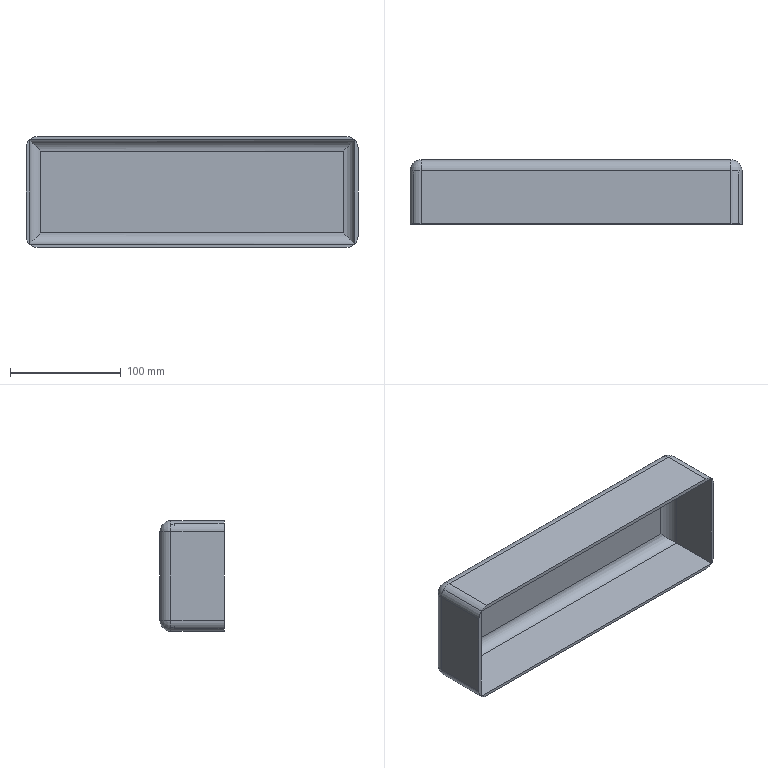Part | STEP file | 301 water tank | 1 solid | 27 faces | box 300 x 58 x 100 mm | volume 214812 mm3 | cylinder 12 | plane 11 | sphere 4 | commonest cylinder face diameters 20 x12